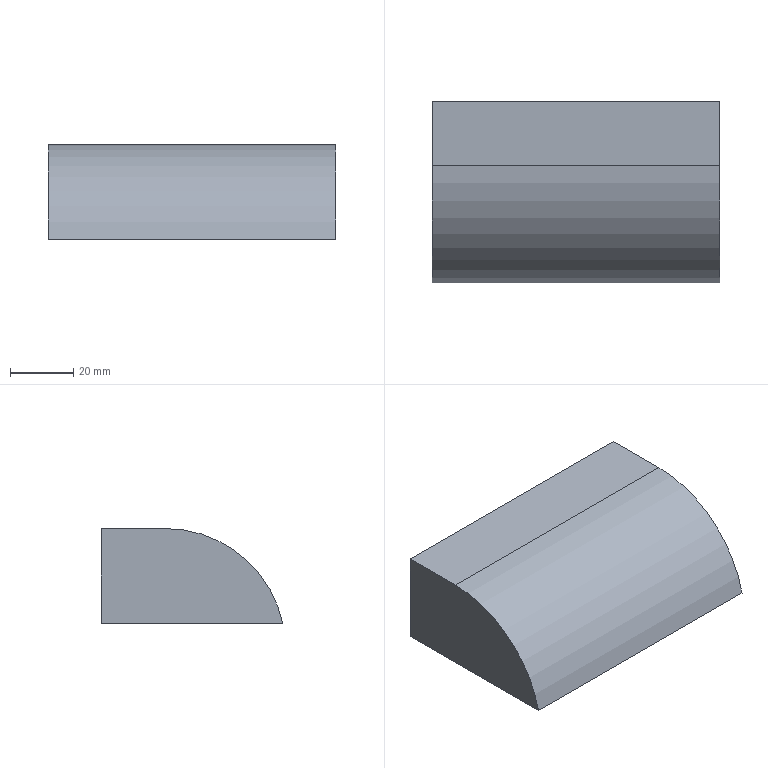Part | SolidWorks | features SweepThread 2, Extrusion 1, Fillet 1, ICE 1 | 1 solid | 66 faces | box 91 x 57.44 x 30 mm | volume 125435 mm3 | cylinder 47 | plane 11 | spline 8 | commonest cylinder face diameters 12 x46 76 x1